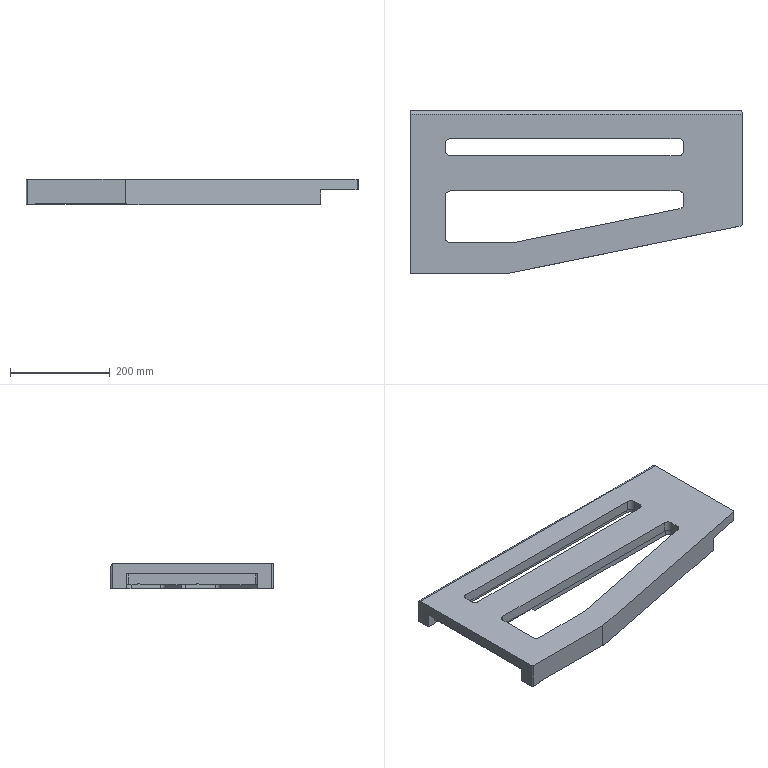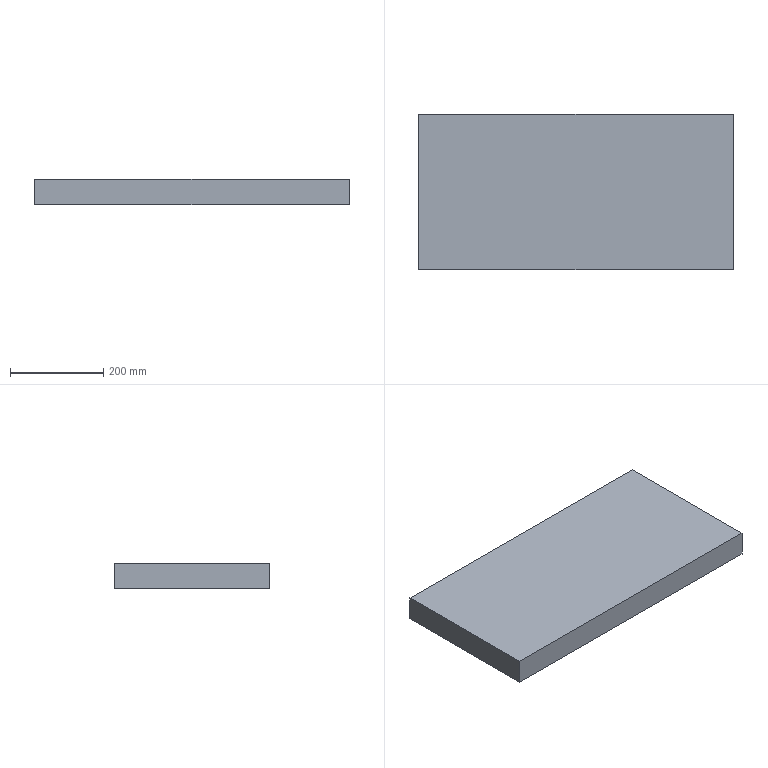CAM job | NX | 3-axis milling | part box 667 x 326 x 51 mm | stock box 675 x 334 x 55 mm
Tools:
number,name,description,diameter,corner_radius,flute_length,length,flutes
4,D40R0.8,Milling Tool-5 Parameters,40.0,0.8,50.0,75.0,2
6,D16R0.8,Milling Tool-5 Parameters,16.0,0.8,50.0,75.0,2
7,D6A45,Milling Tool-5 Parameters,6.0,0.0,3.0,3.0,2
1,D63R0.8,Milling Tool-5 Parameters,63.0,0.8,50.0,75.0,2
3,D30R0.8,Milling Tool-5 Parameters,30.0,0.8,50.0,75.0,2
10,R5,Milling Tool-5 Parameters,10.0,5.0,50.0,75.0,2
Operations:
program,operation,operation_type,tool,method,geometry_group,spindle_rpm,surface_speed,feed_per_tooth,feed_cut,feed_plunge,cut_length_mm,path_length_mm,cut_time_min,machine_time_min
1压外面,ZLEVEL_PROFILE,ZLevelMilling,D40R0.8,METHOD,A,1300.0,163.0,0.7692,2000.0,1000.0,220233.599,220674.012,110.152,110.196
1压外面,ZLEVEL_PROFILE_COPY,ZLevelMilling,D16R0.8,METHOD,A,2000.0,100.0,0.5,2000.0,1000.0,177786.472,178334.654,88.927,88.981
1压外面,ZLEVEL_PROFILE_COPY_1,ZLevelMilling,D16R0.8,METHOD,A,2000.0,100.0,0.5,2000.0,1000.0,42483.517,66883.666,24.518,26.958
1压外面,ZLEVEL_PROFILE_COPY_1_COPY_COPY_COPY_COPY_2_COPY,ZLevelMilling,D6A45,METHOD,A,4000.0,75.0,0.125,1000.0,1000.0,2092.885,2978,2.093,2.181
1压内面,FLOOR_WALL,VolumeBased25DMillingOperation,D63R0.8,METHOD,A,1200.0,237.0,0.5,1200.0,100.0,92152.076,94178.249,76.793,76.996
1压内面,FLOOR_WALL_COPY_2,VolumeBased25DMillingOperation,D63R0.8,METHOD,A,2000.0,395.0,0.3,1200.0,100.0,5229.719,5363.619,4.358,4.372
1压内面,ZLEVEL_PROFILE_COPY_COPY,ZLevelMilling,D30R0.8,METHOD,A,1500.0,150.0,0.6667,2000.0,1000.0,298710.853,298899.853,149.373,149.392
1压内面,FLOOR_WALL_COPY,VolumeBased25DMillingOperation,D63R0.8,METHOD,A,1200.0,237.0,0.5,1200.0,100.0,80405.832,118121.823,67.005,70.776
1压内面,FLOOR_WALL_COPY_COPY_1,VolumeBased25DMillingOperation,D63R0.8,METHOD,A,2000.0,395.0,0.3,1200.0,100.0,934.952,1128.851,0.7791,0.7985
1压内面,FLOOR_WALL_COPY_COPY,VolumeBased25DMillingOperation,D30R0.8,METHOD,A,2000.0,188.0,0.3,1200.0,100.0,3844.8,4298.4,3.204,3.249
1压内面,FLOOR_WALL_COPY_COPY_COPY,VolumeBased25DMillingOperation,D30R0.8,METHOD,A,2000.0,188.0,0.3,1200.0,100.0,5598.173,6838.523,4.665,4.789
1压内面,FLOOR_WALL_COPY_COPY_COPY_COPY,VolumeBased25DMillingOperation,D30R0.8,METHOD,A,2000.0,188.0,0.3,1200.0,100.0,37318.524,40586.724,31.099,31.426
1压内面,FLOOR_WALL_COPY_COPY_COPY_COPY_COPY,VolumeBased25DMillingOperation,D30R0.8,METHOD,A,2000.0,395.0,0.3,1200.0,100.0,1515,1664.9,1.262,1.278
1压内面,FLOOR_WALL_1,VolumeBased25DMillingOperation,D30R0.8,METHOD,A,1500.0,150.0,0.6667,2000.0,100.0,18011.7,32685.615,9.006,10.473
1压内面,FLOOR_WALL_1_COPY,VolumeBased25DMillingOperation,D30R0.8,METHOD,A,2300.0,216.0,0.2609,1200.0,100.0,285.9,479.8,0.2383,0.2576
1压内面,ZLEVEL_PROFILE_COPY_1_COPY,ZLevelMilling,D16R0.8,METHOD,A,2000.0,100.0,0.5,2000.0,1000.0,5654.033,8962.139,3.354,3.684
1压内面,ZLEVEL_PROFILE_COPY_1_COPY_COPY,ZLevelMilling,D16R0.8,METHOD,A,2000.0,100.0,0.5,2000.0,1000.0,2789.113,2937.205,1.397,1.411
1压内面,FIXED_CONTOUR,SurfaceContour,R5,METHOD,A,5000.0,157.0,0.2,2000.0,1000.0,9963.843,10360.158,4.989,5.029
1压内面,ZLEVEL_PROFILE_COPY_1_COPY_COPY_COPY_COPY_2_COPY_COPY,ZLevelMilling,D6A45,METHOD,A,4000.0,75.0,0.125,1000.0,1000.0,3276.259,3833.006,3.276,3.332
1压内面,ZLEVEL_PROFILE_COPY_1_COPY_COPY_COPY_COPY_2_COPY_COPY_COPY,ZLevelMilling,D6A45,METHOD,A,4000.0,75.0,0.125,1000.0,1000.0,731.669,2620.236,0.7317,0.9205
1压内面,ZLEVEL_PROFILE_COPY_1_COPY_COPY_COPY_COPY_2_COPY_COPY_COPY_COPY,ZLevelMilling,D6A45,METHOD,A,4000.0,75.0,0.125,1000.0,1000.0,649.22,1657.235,0.6492,0.75
2压圈外,FLOOR_WALL_COPY_1,VolumeBased25DMillingOperation,D63R0.8,METHOD,B,1200.0,237.0,0.5,1200.0,100.0,4618.999,4752.899,3.849,3.863
2压圈外,ZLEVEL_PROFILE_COPY_1_COPY_COPY_COPY,ZLevelMilling,D16R0.8,METHOD,B,2000.0,100.0,0.5,2000.0,1000.0,43803.985,43951.995,21.904,21.919
2压圈外,ZLEVEL_PROFILE_COPY_1_COPY_COPY_COPY_COPY_2_COPY_COPY_COPY_1,ZLevelMilling,D6A45,METHOD,B,4000.0,75.0,0.125,1000.0,1000.0,1275.296,2515.158,1.275,1.399
2压圈内,FLOOR_WALL_COPY_1_COPY,VolumeBased25DMillingOperation,D63R0.8,METHOD,B,1200.0,237.0,0.5,1200.0,100.0,3877.951,4011.851,3.232,3.245
2压圈内,ZLEVEL_PROFILE_COPY_1_COPY_COPY_COPY_COPY_2_COPY_COPY_COPY_1_COPY,ZLevelMilling,D6A45,METHOD,B,4000.0,75.0,0.125,1000.0,1000.0,2062.885,2949.452,2.063,2.151